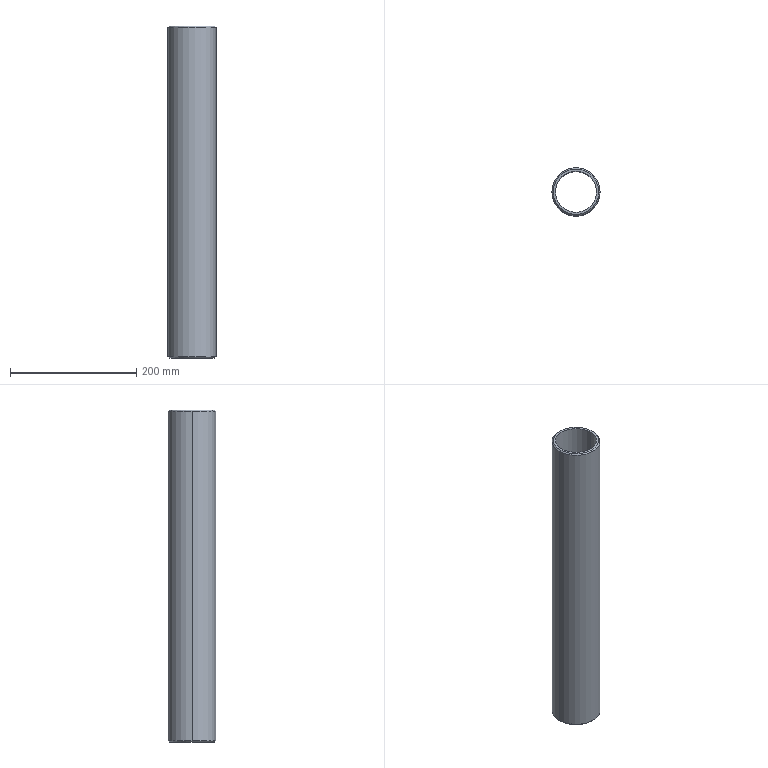Part | SolidWorks | features Chamfer 1, Extrusion 1 | 1 solid | 10 faces | box 76 x 76 x 525 mm | volume 638592 mm3 | cone 4 | cylinder 4 | plane 2 | commonest cylinder face diameters 65 x2 76 x2
STEP:
#1=CARTESIAN_POINT('',(-36.,0.,0.));
#2=VERTEX_POINT('',#1);
#3=CARTESIAN_POINT('',(36.,0.,0.));
#4=VERTEX_POINT('',#3);
#5=CARTESIAN_POINT('',(0.,0.,0.));
#6=DIRECTION('',(0.,0.,-1.));
#7=DIRECTION('',(1.,0.,0.));
#8=AXIS2_PLACEMENT_3D('',#5,#6,#7);
#9=CIRCLE('',#8,36.);
#10=EDGE_CURVE('',#2,#4,#9,.T.);
#11=ORIENTED_EDGE('',*,*,#10,.F.);
#12=CARTESIAN_POINT('',(-38.,0.,2.));
#13=VERTEX_POINT('',#12);
#14=CARTESIAN_POINT('',(-38.,0.,2.));
#15=DIRECTION('',(-0.7071,0.,0.7071));
#16=VECTOR('',#15,1000.);
#17=LINE('',#14,#16);
#18=EDGE_CURVE('',#2,#13,#17,.T.);
#19=ORIENTED_EDGE('',*,*,#18,.T.);
#20=CARTESIAN_POINT('',(38.,0.,2.));
#21=VERTEX_POINT('',#20);
#22=CARTESIAN_POINT('',(0.,0.,2.));
#23=DIRECTION('',(0.,0.,1.));
#24=DIRECTION('',(1.,0.,0.));
#25=AXIS2_PLACEMENT_3D('',#22,#23,#24);
#26=CIRCLE('',#25,38.);
#27=EDGE_CURVE('',#21,#13,#26,.T.);
#28=ORIENTED_EDGE('',*,*,#27,.F.);
#29=CARTESIAN_POINT('',(38.,0.,2.));
#30=DIRECTION('',(0.7071,0.,0.7071));
#31=VECTOR('',#30,1000.);
#32=LINE('',#29,#31);
#33=EDGE_CURVE('',#4,#21,#32,.T.);
#34=ORIENTED_EDGE('',*,*,#33,.F.);
#35=EDGE_LOOP('',(#11,#19,#28,#34));
#36=FACE_OUTER_BOUND('',#35,.T.);
#37=CARTESIAN_POINT('',(0.,0.,2.));
#38=DIRECTION('',(0.,0.,1.));
#39=DIRECTION('',(1.,0.,0.));
#40=AXIS2_PLACEMENT_3D('',#37,#38,#39);
#41=CONICAL_SURFACE('',#40,38.,0.7854);
#42=ADVANCED_FACE('',(#36),#41,.T.);
#43=CARTESIAN_POINT('',(36.,0.,525.));
#44=VERTEX_POINT('',#43);
#45=CARTESIAN_POINT('',(-36.,0.,525.));
#46=VERTEX_POINT('',#45);
#47=CARTESIAN_POINT('',(0.,0.,525.));
#48=DIRECTION('',(0.,0.,1.));
#49=DIRECTION('',(1.,0.,0.));
#50=AXIS2_PLACEMENT_3D('',#47,#48,#49);
#51=CIRCLE('',#50,36.);
#52=EDGE_CURVE('',#44,#46,#51,.T.);
#53=ORIENTED_EDGE('',*,*,#52,.F.);
#54=CARTESIAN_POINT('',(38.,0.,523.));
#55=VERTEX_POINT('',#54);
#56=CARTESIAN_POINT('',(36.,0.,525.));
#57=DIRECTION('',(0.7071,0.,-0.7071));
#58=VECTOR('',#57,1000.);
#59=LINE('',#56,#58);
#60=EDGE_CURVE('',#44,#55,#59,.T.);
#61=ORIENTED_EDGE('',*,*,#60,.T.);
#62=CARTESIAN_POINT('',(-38.,0.,523.));
#63=VERTEX_POINT('',#62);
#64=CARTESIAN_POINT('',(0.,0.,523.));
#65=DIRECTION('',(0.,0.,-1.));
#66=DIRECTION('',(1.,0.,0.));
#67=AXIS2_PLACEMENT_3D('',#64,#65,#66);
#68=CIRCLE('',#67,38.);
#69=EDGE_CURVE('',#63,#55,#68,.T.);
#70=ORIENTED_EDGE('',*,*,#69,.F.);
#71=CARTESIAN_POINT('',(-36.,0.,525.));
#72=DIRECTION('',(-0.7071,0.,-0.7071));
#73=VECTOR('',#72,1000.);
#74=LINE('',#71,#73);
#75=EDGE_CURVE('',#46,#63,#74,.T.);
#76=ORIENTED_EDGE('',*,*,#75,.F.);
#77=EDGE_LOOP('',(#53,#61,#70,#76));
#78=FACE_OUTER_BOUND('',#77,.T.);
#79=CARTESIAN_POINT('',(0.,0.,525.));
#80=DIRECTION('',(0.,0.,-1.));
#81=DIRECTION('',(-1.,0.,0.));
#82=AXIS2_PLACEMENT_3D('',#79,#80,#81);
#83=CONICAL_SURFACE('',#82,36.,0.7854);
#84=ADVANCED_FACE('',(#78),#83,.T.);
#85=CARTESIAN_POINT('',(-32.5,0.,525.));
#86=VERTEX_POINT('',#85);
#87=CARTESIAN_POINT('',(32.5,0.,525.));
#88=VERTEX_POINT('',#87);
#89=CARTESIAN_POINT('',(0.,0.,525.));
#90=DIRECTION('',(0.,0.,1.));
#91=DIRECTION('',(1.,0.,0.));
#92=AXIS2_PLACEMENT_3D('',#89,#90,#91);
#93=CIRCLE('',#92,32.5);
#94=EDGE_CURVE('',#86,#88,#93,.T.);
#95=ORIENTED_EDGE('',*,*,#94,.T.);
#96=CARTESIAN_POINT('',(32.5,0.,0.));
#97=VERTEX_POINT('',#96);
#98=CARTESIAN_POINT('',(32.5,0.,525.));
#99=DIRECTION('',(0.,0.,-1.));
#100=VECTOR('',#99,1000.);
#101=LINE('',#98,#100);
#102=EDGE_CURVE('',#88,#97,#101,.T.);
#103=ORIENTED_EDGE('',*,*,#102,.T.);
#104=CARTESIAN_POINT('',(-32.5,0.,0.));
#105=VERTEX_POINT('',#104);
#106=CARTESIAN_POINT('',(0.,0.,0.));
#107=DIRECTION('',(0.,0.,1.));
#108=DIRECTION('',(1.,0.,0.));
#109=AXIS2_PLACEMENT_3D('',#106,#107,#108);
#110=CIRCLE('',#109,32.5);
#111=EDGE_CURVE('',#105,#97,#110,.T.);
#112=ORIENTED_EDGE('',*,*,#111,.F.);
#113=CARTESIAN_POINT('',(-32.5,0.,525.));
#114=DIRECTION('',(0.,0.,-1.));
#115=VECTOR('',#114,1000.);
#116=LINE('',#113,#115);
#117=EDGE_CURVE('',#86,#105,#116,.T.);
#118=ORIENTED_EDGE('',*,*,#117,.F.);
#119=EDGE_LOOP('',(#95,#103,#112,#118));
#120=FACE_OUTER_BOUND('',#119,.T.);
#121=CARTESIAN_POINT('',(0.,0.,525.));
#122=DIRECTION('',(0.,0.,-1.));
#123=DIRECTION('',(-1.,0.,0.));
#124=AXIS2_PLACEMENT_3D('',#121,#122,#123);
#125=CYLINDRICAL_SURFACE('',#124,32.5);
#126=ADVANCED_FACE('',(#120),#125,.F.);
#127=ORIENTED_EDGE('',*,*,#69,.T.);
#128=CARTESIAN_POINT('',(38.,0.,525.));
#129=DIRECTION('',(0.,0.,-1.));
#130=VECTOR('',#129,1000.);
#131=LINE('',#128,#130);
#132=EDGE_CURVE('',#55,#21,#131,.T.);
#133=ORIENTED_EDGE('',*,*,#132,.T.);
#134=ORIENTED_EDGE('',*,*,#27,.T.);
#135=CARTESIAN_POINT('',(-38.,0.,525.));
#136=DIRECTION('',(0.,0.,-1.));
#137=VECTOR('',#136,1000.);
#138=LINE('',#135,#137);
#139=EDGE_CURVE('',#63,#13,#138,.T.);
#140=ORIENTED_EDGE('',*,*,#139,.F.);
#141=EDGE_LOOP('',(#127,#133,#134,#140));
#142=FACE_OUTER_BOUND('',#141,.T.);
#143=CARTESIAN_POINT('',(0.,0.,525.));
#144=DIRECTION('',(0.,0.,-1.));
#145=DIRECTION('',(-1.,0.,0.));
#146=AXIS2_PLACEMENT_3D('',#143,#144,#145);
#147=CYLINDRICAL_SURFACE('',#146,38.);
#148=ADVANCED_FACE('',(#142),#147,.T.);
#149=CARTESIAN_POINT('',(0.,0.,525.));
#150=DIRECTION('',(0.,0.,1.));
#151=DIRECTION('',(1.,0.,0.));
#152=AXIS2_PLACEMENT_3D('',#149,#150,#151);
#153=CIRCLE('',#152,36.);
#154=EDGE_CURVE('',#46,#44,#153,.T.);
#155=ORIENTED_EDGE('',*,*,#154,.T.);
#156=ORIENTED_EDGE('',*,*,#52,.T.);
#157=EDGE_LOOP('',(#155,#156));
#158=FACE_OUTER_BOUND('',#157,.T.);
#159=ORIENTED_EDGE('',*,*,#94,.F.);
#160=CARTESIAN_POINT('',(0.,0.,525.));
#161=DIRECTION('',(0.,0.,1.));
#162=DIRECTION('',(1.,0.,0.));
#163=AXIS2_PLACEMENT_3D('',#160,#161,#162);
#164=CIRCLE('',#163,32.5);
#165=EDGE_CURVE('',#88,#86,#164,.T.);
#166=ORIENTED_EDGE('',*,*,#165,.F.);
#167=EDGE_LOOP('',(#159,#166));
#168=FACE_BOUND('',#167,.T.);
#169=CARTESIAN_POINT('',(0.,0.,525.));
#170=DIRECTION('',(0.,0.,1.));
#171=DIRECTION('',(1.,0.,0.));
#172=AXIS2_PLACEMENT_3D('',#169,#170,#171);
#173=PLANE('',#172);
#174=ADVANCED_FACE('',(#158,#168),#173,.T.);
#175=CARTESIAN_POINT('',(0.,0.,0.));
#176=DIRECTION('',(0.,0.,-1.));
#177=DIRECTION('',(1.,0.,0.));
#178=AXIS2_PLACEMENT_3D('',#175,#176,#177);
#179=CIRCLE('',#178,36.);
#180=EDGE_CURVE('',#4,#2,#179,.T.);
#181=ORIENTED_EDGE('',*,*,#180,.T.);
#182=ORIENTED_EDGE('',*,*,#10,.T.);
#183=EDGE_LOOP('',(#181,#182));
#184=FACE_OUTER_BOUND('',#183,.T.);
#185=ORIENTED_EDGE('',*,*,#111,.T.);
#186=CARTESIAN_POINT('',(0.,0.,0.));
#187=DIRECTION('',(0.,0.,1.));
#188=DIRECTION('',(1.,0.,0.));
#189=AXIS2_PLACEMENT_3D('',#186,#187,#188);
#190=CIRCLE('',#189,32.5);
#191=EDGE_CURVE('',#97,#105,#190,.T.);
#192=ORIENTED_EDGE('',*,*,#191,.T.);
#193=EDGE_LOOP('',(#185,#192));
#194=FACE_BOUND('',#193,.T.);
#195=CARTESIAN_POINT('',(0.,0.,0.));
#196=DIRECTION('',(0.,0.,1.));
#197=DIRECTION('',(1.,0.,0.));
#198=AXIS2_PLACEMENT_3D('',#195,#196,#197);
#199=PLANE('',#198);
#200=ADVANCED_FACE('',(#184,#194),#199,.F.);
#201=ORIENTED_EDGE('',*,*,#132,.F.);
#202=CARTESIAN_POINT('',(0.,0.,523.));
#203=DIRECTION('',(0.,0.,-1.));
#204=DIRECTION('',(1.,0.,0.));
#205=AXIS2_PLACEMENT_3D('',#202,#203,#204);
#206=CIRCLE('',#205,38.);
#207=EDGE_CURVE('',#55,#63,#206,.T.);
#208=ORIENTED_EDGE('',*,*,#207,.T.);
#209=ORIENTED_EDGE('',*,*,#139,.T.);
#210=CARTESIAN_POINT('',(0.,0.,2.));
#211=DIRECTION('',(0.,0.,1.));
#212=DIRECTION('',(1.,0.,0.));
#213=AXIS2_PLACEMENT_3D('',#210,#211,#212);
#214=CIRCLE('',#213,38.);
#215=EDGE_CURVE('',#13,#21,#214,.T.);
#216=ORIENTED_EDGE('',*,*,#215,.T.);
#217=EDGE_LOOP('',(#201,#208,#209,#216));
#218=FACE_OUTER_BOUND('',#217,.T.);
#219=CARTESIAN_POINT('',(0.,0.,525.));
#220=DIRECTION('',(0.,0.,-1.));
#221=DIRECTION('',(-1.,0.,0.));
#222=AXIS2_PLACEMENT_3D('',#219,#220,#221);
#223=CYLINDRICAL_SURFACE('',#222,38.);
#224=ADVANCED_FACE('',(#218),#223,.T.);
#225=ORIENTED_EDGE('',*,*,#102,.F.);
#226=ORIENTED_EDGE('',*,*,#165,.T.);
#227=ORIENTED_EDGE('',*,*,#117,.T.);
#228=ORIENTED_EDGE('',*,*,#191,.F.);
#229=EDGE_LOOP('',(#225,#226,#227,#228));
#230=FACE_OUTER_BOUND('',#229,.T.);
#231=CARTESIAN_POINT('',(0.,0.,525.));
#232=DIRECTION('',(0.,0.,-1.));
#233=DIRECTION('',(-1.,0.,0.));
#234=AXIS2_PLACEMENT_3D('',#231,#232,#233);
#235=CYLINDRICAL_SURFACE('',#234,32.5);
#236=ADVANCED_FACE('',(#230),#235,.F.);
#237=ORIENTED_EDGE('',*,*,#60,.F.);
#238=ORIENTED_EDGE('',*,*,#154,.F.);
#239=ORIENTED_EDGE('',*,*,#75,.T.);
#240=ORIENTED_EDGE('',*,*,#207,.F.);
#241=EDGE_LOOP('',(#237,#238,#239,#240));
#242=FACE_OUTER_BOUND('',#241,.T.);
#243=CARTESIAN_POINT('',(0.,0.,525.));
#244=DIRECTION('',(0.,0.,-1.));
#245=DIRECTION('',(-1.,0.,0.));
#246=AXIS2_PLACEMENT_3D('',#243,#244,#245);
#247=CONICAL_SURFACE('',#246,36.,0.7854);
#248=ADVANCED_FACE('',(#242),#247,.T.);
#249=ORIENTED_EDGE('',*,*,#18,.F.);
#250=ORIENTED_EDGE('',*,*,#180,.F.);
#251=ORIENTED_EDGE('',*,*,#33,.T.);
#252=ORIENTED_EDGE('',*,*,#215,.F.);
#253=EDGE_LOOP('',(#249,#250,#251,#252));
#254=FACE_OUTER_BOUND('',#253,.T.);
#255=CARTESIAN_POINT('',(0.,0.,2.));
#256=DIRECTION('',(0.,0.,1.));
#257=DIRECTION('',(1.,0.,0.));
#258=AXIS2_PLACEMENT_3D('',#255,#256,#257);
#259=CONICAL_SURFACE('',#258,38.,0.7854);
#260=ADVANCED_FACE('',(#254),#259,.T.);
#261=CLOSED_SHELL('',(#42,#84,#126,#148,#174,#200,#224,#236,#248,#260));
#262=MANIFOLD_SOLID_BREP('',#261);
#263=CARTESIAN_POINT('',(0.,0.,0.));
#264=DIRECTION('',(0.,0.,1.));
#265=DIRECTION('',(1.,0.,0.));
#266=AXIS2_PLACEMENT_3D('',#263,#264,#265);
#267=(LENGTH_UNIT()NAMED_UNIT(*)SI_UNIT(.MILLI.,.METRE.));
#268=UNCERTAINTY_MEASURE_WITH_UNIT(LENGTH_MEASURE(0.00001),#267,'','');
#269=(NAMED_UNIT(*)PLANE_ANGLE_UNIT()SI_UNIT($,.RADIAN.));
#270=(NAMED_UNIT(*)SI_UNIT($,.STERADIAN.)SOLID_ANGLE_UNIT());
#271=(GEOMETRIC_REPRESENTATION_CONTEXT(3)GLOBAL_UNCERTAINTY_ASSIGNED_CONTEXT((#268))GLOBAL_UNIT_ASSIGNED_CONTEXT((#267,#269,#270))REPRESENTATION_CONTEXT('',''));
#272=ADVANCED_BREP_SHAPE_REPRESENTATION('',(#262,#266),#271);